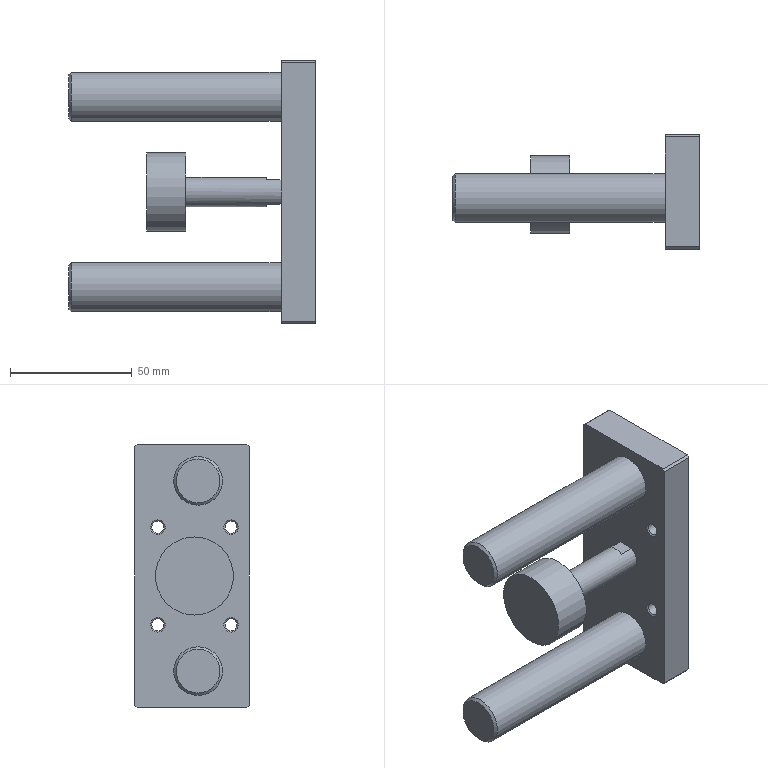Part | NX | features BREP 1 | 1 solid | 98 faces | box 101 x 47 x 108 mm | volume 140081 mm3 | cylinder 54 | plane 31 | cone 10 | torus 3 | commonest cylinder face diameters 1.589 x18 2.781 x18 4.917 x4 9 x4 13 x3 15 x3